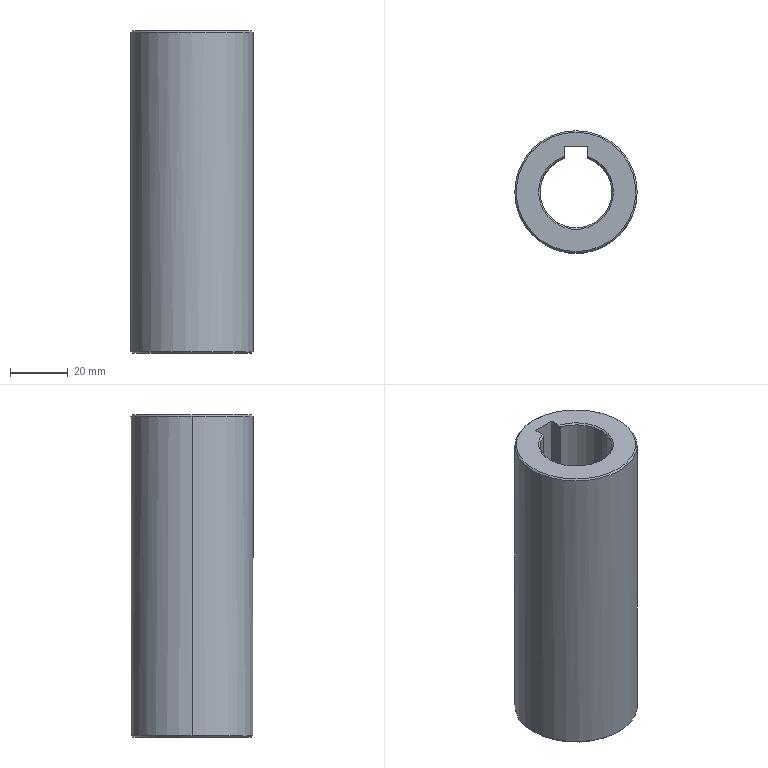Part | STEP file | Output hollow shaft_063_25.step_1 | 1 solid | 18 faces | box 42.5 x 42.5 x 112 mm | volume 100706 mm3 | cone 8 | cylinder 5 | plane 5 | commonest cylinder face diameters 25 x3 42.5 x2
STEP:
#1=CARTESIAN_POINT('',(0.,0.,0.));
#2=DIRECTION('',(0.,0.,1.));
#3=DIRECTION('',(1.,0.,0.));
#4=AXIS2_PLACEMENT_3D('',#1,#2,#3);
#5=CARTESIAN_POINT('',(21.25,0.,-55.5));
#6=VERTEX_POINT('',#5);
#7=CARTESIAN_POINT('',(-21.25,0.,-55.5));
#8=VERTEX_POINT('',#7);
#9=CARTESIAN_POINT('',(0.,0.,-55.5));
#10=DIRECTION('',(0.,0.,1.));
#11=DIRECTION('',(1.,0.,0.));
#12=AXIS2_PLACEMENT_3D('',#9,#10,#11);
#13=CIRCLE('',#12,21.25);
#14=CARTESIAN_POINT('',(0.,0.,92.725));
#15=DIRECTION('',(0.,0.,1.));
#16=DIRECTION('',(1.,0.,0.));
#17=AXIS2_PLACEMENT_3D('',#14,#15,#16);
#18=CYLINDRICAL_SURFACE('',#17,21.25);
#19=CARTESIAN_POINT('',(0.,-148.225));
#20=DIRECTION('',(1.,0.));
#21=VECTOR('',#20,1.);
#22=LINE('',#19,#21);
#23=(GEOMETRIC_REPRESENTATION_CONTEXT(2)PARAMETRIC_REPRESENTATION_CONTEXT()REPRESENTATION_CONTEXT('',''));
#24=DEFINITIONAL_REPRESENTATION('',(#22),#23);
#25=PCURVE('',#18,#24);
#26=CARTESIAN_POINT('',(0.,0.,-55.5));
#27=DIRECTION('',(0.,0.,1.));
#28=DIRECTION('',(1.,0.,0.));
#29=AXIS2_PLACEMENT_3D('',#26,#27,#28);
#30=CONICAL_SURFACE('',#29,21.25,0.7854);
#31=CARTESIAN_POINT('',(0.,0.));
#32=DIRECTION('',(1.,0.));
#33=VECTOR('',#32,1.);
#34=LINE('',#31,#33);
#35=(GEOMETRIC_REPRESENTATION_CONTEXT(2)PARAMETRIC_REPRESENTATION_CONTEXT()REPRESENTATION_CONTEXT('',''));
#36=DEFINITIONAL_REPRESENTATION('',(#34),#35);
#37=PCURVE('',#30,#36);
#38=SURFACE_CURVE('',#13,(#25,#37),.PCURVE_S1.);
#39=EDGE_CURVE('',#6,#8,#38,.T.);
#40=ORIENTED_EDGE('',*,*,#39,.T.);
#41=CARTESIAN_POINT('',(-21.25,0.,55.5));
#42=VERTEX_POINT('',#41);
#43=CARTESIAN_POINT('',(-21.25,0.,92.725));
#44=DIRECTION('',(0.,0.,1.));
#45=VECTOR('',#44,1.);
#46=LINE('',#43,#45);
#47=CARTESIAN_POINT('',(3.142,0.));
#48=DIRECTION('',(0.,1.));
#49=VECTOR('',#48,1.);
#50=LINE('',#47,#49);
#51=(GEOMETRIC_REPRESENTATION_CONTEXT(2)PARAMETRIC_REPRESENTATION_CONTEXT()REPRESENTATION_CONTEXT('',''));
#52=DEFINITIONAL_REPRESENTATION('',(#50),#51);
#53=PCURVE('',#18,#52);
#54=CARTESIAN_POINT('',(0.,0.,92.725));
#55=DIRECTION('',(0.,0.,1.));
#56=DIRECTION('',(1.,0.,0.));
#57=AXIS2_PLACEMENT_3D('',#54,#55,#56);
#58=CYLINDRICAL_SURFACE('',#57,21.25);
#59=CARTESIAN_POINT('',(3.142,0.));
#60=DIRECTION('',(0.,1.));
#61=VECTOR('',#60,1.);
#62=LINE('',#59,#61);
#63=(GEOMETRIC_REPRESENTATION_CONTEXT(2)PARAMETRIC_REPRESENTATION_CONTEXT()REPRESENTATION_CONTEXT('',''));
#64=DEFINITIONAL_REPRESENTATION('',(#62),#63);
#65=PCURVE('',#58,#64);
#66=SURFACE_CURVE('',#46,(#53,#65),.PCURVE_S1.);
#67=EDGE_CURVE('',#8,#42,#66,.T.);
#68=ORIENTED_EDGE('',*,*,#67,.T.);
#69=CARTESIAN_POINT('',(0.,21.25,55.5));
#70=VERTEX_POINT('',#69);
#71=CARTESIAN_POINT('',(0.,0.,55.5));
#72=DIRECTION('',(0.,0.,-1.));
#73=DIRECTION('',(1.,0.,0.));
#74=AXIS2_PLACEMENT_3D('',#71,#72,#73);
#75=CIRCLE('',#74,21.25);
#76=CARTESIAN_POINT('',(6.283,-37.225));
#77=DIRECTION('',(-1.,0.));
#78=VECTOR('',#77,1.);
#79=LINE('',#76,#78);
#80=(GEOMETRIC_REPRESENTATION_CONTEXT(2)PARAMETRIC_REPRESENTATION_CONTEXT()REPRESENTATION_CONTEXT('',''));
#81=DEFINITIONAL_REPRESENTATION('',(#79),#80);
#82=PCURVE('',#18,#81);
#83=CARTESIAN_POINT('',(0.,0.,55.5));
#84=DIRECTION('',(0.,0.,-1.));
#85=DIRECTION('',(0.,1.,0.));
#86=AXIS2_PLACEMENT_3D('',#83,#84,#85);
#87=CONICAL_SURFACE('',#86,21.25,0.7854);
#88=CARTESIAN_POINT('',(1.571,0.));
#89=DIRECTION('',(1.,0.));
#90=VECTOR('',#89,1.);
#91=LINE('',#88,#90);
#92=(GEOMETRIC_REPRESENTATION_CONTEXT(2)PARAMETRIC_REPRESENTATION_CONTEXT()REPRESENTATION_CONTEXT('',''));
#93=DEFINITIONAL_REPRESENTATION('',(#91),#92);
#94=PCURVE('',#87,#93);
#95=SURFACE_CURVE('',#75,(#82,#94),.PCURVE_S1.);
#96=EDGE_CURVE('',#42,#70,#95,.T.);
#97=ORIENTED_EDGE('',*,*,#96,.T.);
#98=CARTESIAN_POINT('',(21.25,0.,55.5));
#99=VERTEX_POINT('',#98);
#100=CARTESIAN_POINT('',(0.,0.,55.5));
#101=DIRECTION('',(0.,0.,-1.));
#102=DIRECTION('',(1.,0.,0.));
#103=AXIS2_PLACEMENT_3D('',#100,#101,#102);
#104=CIRCLE('',#103,21.25);
#105=CARTESIAN_POINT('',(6.283,-37.225));
#106=DIRECTION('',(-1.,0.));
#107=VECTOR('',#106,1.);
#108=LINE('',#105,#107);
#109=(GEOMETRIC_REPRESENTATION_CONTEXT(2)PARAMETRIC_REPRESENTATION_CONTEXT()REPRESENTATION_CONTEXT('',''));
#110=DEFINITIONAL_REPRESENTATION('',(#108),#109);
#111=PCURVE('',#18,#110);
#112=CARTESIAN_POINT('',(0.,0.,55.5));
#113=DIRECTION('',(0.,0.,-1.));
#114=DIRECTION('',(0.,1.,0.));
#115=AXIS2_PLACEMENT_3D('',#112,#113,#114);
#116=CONICAL_SURFACE('',#115,21.25,0.7854);
#117=CARTESIAN_POINT('',(-4.712,0.));
#118=DIRECTION('',(1.,0.));
#119=VECTOR('',#118,1.);
#120=LINE('',#117,#119);
#121=(GEOMETRIC_REPRESENTATION_CONTEXT(2)PARAMETRIC_REPRESENTATION_CONTEXT()REPRESENTATION_CONTEXT('',''));
#122=DEFINITIONAL_REPRESENTATION('',(#120),#121);
#123=PCURVE('',#116,#122);
#124=SURFACE_CURVE('',#104,(#111,#123),.PCURVE_S1.);
#125=EDGE_CURVE('',#70,#99,#124,.T.);
#126=ORIENTED_EDGE('',*,*,#125,.T.);
#127=CARTESIAN_POINT('',(21.25,0.,92.725));
#128=DIRECTION('',(0.,0.,1.));
#129=VECTOR('',#128,1.);
#130=LINE('',#127,#129);
#131=CARTESIAN_POINT('',(0.,0.));
#132=DIRECTION('',(0.,1.));
#133=VECTOR('',#132,1.);
#134=LINE('',#131,#133);
#135=(GEOMETRIC_REPRESENTATION_CONTEXT(2)PARAMETRIC_REPRESENTATION_CONTEXT()REPRESENTATION_CONTEXT('',''));
#136=DEFINITIONAL_REPRESENTATION('',(#134),#135);
#137=PCURVE('',#18,#136);
#138=CARTESIAN_POINT('',(6.283,0.));
#139=DIRECTION('',(0.,1.));
#140=VECTOR('',#139,1.);
#141=LINE('',#138,#140);
#142=(GEOMETRIC_REPRESENTATION_CONTEXT(2)PARAMETRIC_REPRESENTATION_CONTEXT()REPRESENTATION_CONTEXT('',''));
#143=DEFINITIONAL_REPRESENTATION('',(#141),#142);
#144=PCURVE('',#58,#143);
#145=SURFACE_CURVE('',#130,(#137,#144),.PCURVE_S1.);
#146=EDGE_CURVE('',#6,#99,#145,.T.);
#147=ORIENTED_EDGE('',*,*,#146,.F.);
#148=EDGE_LOOP('',(#40,#68,#97,#126,#147));
#149=FACE_BOUND('',#148,.T.);
#150=ADVANCED_FACE('',(#149),#18,.T.);
#151=CARTESIAN_POINT('',(0.,20.75,56.));
#152=VERTEX_POINT('',#151);
#153=CARTESIAN_POINT('',(0.,-20.75,56.));
#154=VERTEX_POINT('',#153);
#155=CARTESIAN_POINT('',(0.,0.,56.));
#156=DIRECTION('',(0.,0.,-1.));
#157=DIRECTION('',(0.,1.,0.));
#158=AXIS2_PLACEMENT_3D('',#155,#156,#157);
#159=CIRCLE('',#158,20.75);
#160=CARTESIAN_POINT('',(0.,-0.5));
#161=DIRECTION('',(1.,0.));
#162=VECTOR('',#161,1.);
#163=LINE('',#160,#162);
#164=(GEOMETRIC_REPRESENTATION_CONTEXT(2)PARAMETRIC_REPRESENTATION_CONTEXT()REPRESENTATION_CONTEXT('',''));
#165=DEFINITIONAL_REPRESENTATION('',(#163),#164);
#166=PCURVE('',#116,#165);
#167=CARTESIAN_POINT('',(0.,13.,56.));
#168=DIRECTION('',(0.,0.,-1.));
#169=DIRECTION('',(-1.,0.,0.));
#170=AXIS2_PLACEMENT_3D('',#167,#168,#169);
#171=PLANE('',#170);
#172=CARTESIAN_POINT('',(0.,-13.));
#173=DIRECTION('',(0.,1.));
#174=AXIS2_PLACEMENT_2D('',#172,#173);
#175=CIRCLE('',#174,20.75);
#176=(GEOMETRIC_REPRESENTATION_CONTEXT(2)PARAMETRIC_REPRESENTATION_CONTEXT()REPRESENTATION_CONTEXT('',''));
#177=DEFINITIONAL_REPRESENTATION('',(#175),#176);
#178=PCURVE('',#171,#177);
#179=SURFACE_CURVE('',#159,(#166,#178),.PCURVE_S1.);
#180=EDGE_CURVE('',#152,#154,#179,.T.);
#181=ORIENTED_EDGE('',*,*,#180,.T.);
#182=CARTESIAN_POINT('',(0.,-21.25,55.5));
#183=VERTEX_POINT('',#182);
#184=CARTESIAN_POINT('',(0.,-21.25,55.5));
#185=DIRECTION('',(0.,-0.7071,-0.7071));
#186=VECTOR('',#185,1.);
#187=LINE('',#184,#186);
#188=CARTESIAN_POINT('',(3.142,0.));
#189=DIRECTION('',(0.,1.));
#190=VECTOR('',#189,1.);
#191=LINE('',#188,#190);
#192=(GEOMETRIC_REPRESENTATION_CONTEXT(2)PARAMETRIC_REPRESENTATION_CONTEXT()REPRESENTATION_CONTEXT('',''));
#193=DEFINITIONAL_REPRESENTATION('',(#191),#192);
#194=PCURVE('',#116,#193);
#195=CARTESIAN_POINT('',(3.142,0.));
#196=DIRECTION('',(0.,1.));
#197=VECTOR('',#196,1.);
#198=LINE('',#195,#197);
#199=(GEOMETRIC_REPRESENTATION_CONTEXT(2)PARAMETRIC_REPRESENTATION_CONTEXT()REPRESENTATION_CONTEXT('',''));
#200=DEFINITIONAL_REPRESENTATION('',(#198),#199);
#201=PCURVE('',#87,#200);
#202=SURFACE_CURVE('',#187,(#194,#201),.PCURVE_S1.);
#203=EDGE_CURVE('',#154,#183,#202,.T.);
#204=ORIENTED_EDGE('',*,*,#203,.T.);
#205=CARTESIAN_POINT('',(0.,0.,55.5));
#206=DIRECTION('',(0.,0.,-1.));
#207=DIRECTION('',(1.,0.,0.));
#208=AXIS2_PLACEMENT_3D('',#205,#206,#207);
#209=CIRCLE('',#208,21.25);
#210=CARTESIAN_POINT('',(1.571,0.));
#211=DIRECTION('',(1.,0.));
#212=VECTOR('',#211,1.);
#213=LINE('',#210,#212);
#214=(GEOMETRIC_REPRESENTATION_CONTEXT(2)PARAMETRIC_REPRESENTATION_CONTEXT()REPRESENTATION_CONTEXT('',''));
#215=DEFINITIONAL_REPRESENTATION('',(#213),#214);
#216=PCURVE('',#116,#215);
#217=CARTESIAN_POINT('',(6.283,-37.225));
#218=DIRECTION('',(-1.,0.));
#219=VECTOR('',#218,1.);
#220=LINE('',#217,#219);
#221=(GEOMETRIC_REPRESENTATION_CONTEXT(2)PARAMETRIC_REPRESENTATION_CONTEXT()REPRESENTATION_CONTEXT('',''));
#222=DEFINITIONAL_REPRESENTATION('',(#220),#221);
#223=PCURVE('',#58,#222);
#224=SURFACE_CURVE('',#209,(#216,#223),.PCURVE_S1.);
#225=EDGE_CURVE('',#99,#183,#224,.T.);
#226=ORIENTED_EDGE('',*,*,#225,.F.);
#227=ORIENTED_EDGE('',*,*,#125,.F.);
#228=CARTESIAN_POINT('',(0.,21.25,55.5));
#229=DIRECTION('',(0.,0.7071,-0.7071));
#230=VECTOR('',#229,1.);
#231=LINE('',#228,#230);
#232=CARTESIAN_POINT('',(0.,0.));
#233=DIRECTION('',(0.,1.));
#234=VECTOR('',#233,1.);
#235=LINE('',#232,#234);
#236=(GEOMETRIC_REPRESENTATION_CONTEXT(2)PARAMETRIC_REPRESENTATION_CONTEXT()REPRESENTATION_CONTEXT('',''));
#237=DEFINITIONAL_REPRESENTATION('',(#235),#236);
#238=PCURVE('',#116,#237);
#239=CARTESIAN_POINT('',(6.283,0.));
#240=DIRECTION('',(0.,1.));
#241=VECTOR('',#240,1.);
#242=LINE('',#239,#241);
#243=(GEOMETRIC_REPRESENTATION_CONTEXT(2)PARAMETRIC_REPRESENTATION_CONTEXT()REPRESENTATION_CONTEXT('',''));
#244=DEFINITIONAL_REPRESENTATION('',(#242),#243);
#245=PCURVE('',#87,#244);
#246=SURFACE_CURVE('',#231,(#238,#245),.PCURVE_S1.);
#247=EDGE_CURVE('',#152,#70,#246,.T.);
#248=ORIENTED_EDGE('',*,*,#247,.F.);
#249=EDGE_LOOP('',(#181,#204,#226,#227,#248));
#250=FACE_BOUND('',#249,.T.);
#251=ADVANCED_FACE('',(#250),#116,.T.);
#252=CARTESIAN_POINT('',(20.75,0.,-56.));
#253=VERTEX_POINT('',#252);
#254=CARTESIAN_POINT('',(-20.75,0.,-56.));
#255=VERTEX_POINT('',#254);
#256=CARTESIAN_POINT('',(0.,0.,-56.));
#257=DIRECTION('',(0.,0.,1.));
#258=DIRECTION('',(1.,0.,0.));
#259=AXIS2_PLACEMENT_3D('',#256,#257,#258);
#260=CIRCLE('',#259,20.75);
#261=CARTESIAN_POINT('',(0.,-0.5));
#262=DIRECTION('',(1.,0.));
#263=VECTOR('',#262,1.);
#264=LINE('',#261,#263);
#265=(GEOMETRIC_REPRESENTATION_CONTEXT(2)PARAMETRIC_REPRESENTATION_CONTEXT()REPRESENTATION_CONTEXT('',''));
#266=DEFINITIONAL_REPRESENTATION('',(#264),#265);
#267=PCURVE('',#30,#266);
#268=CARTESIAN_POINT('',(0.,20.75,-56.));
#269=DIRECTION('',(0.,0.,1.));
#270=DIRECTION('',(1.,0.,0.));
#271=AXIS2_PLACEMENT_3D('',#268,#269,#270);
#272=PLANE('',#271);
#273=CARTESIAN_POINT('',(0.,-20.75));
#274=DIRECTION('',(1.,0.));
#275=AXIS2_PLACEMENT_2D('',#273,#274);
#276=CIRCLE('',#275,20.75);
#277=(GEOMETRIC_REPRESENTATION_CONTEXT(2)PARAMETRIC_REPRESENTATION_CONTEXT()REPRESENTATION_CONTEXT('',''));
#278=DEFINITIONAL_REPRESENTATION('',(#276),#277);
#279=PCURVE('',#272,#278);
#280=SURFACE_CURVE('',#260,(#267,#279),.PCURVE_S1.);
#281=EDGE_CURVE('',#253,#255,#280,.T.);
#282=ORIENTED_EDGE('',*,*,#281,.T.);
#283=CARTESIAN_POINT('',(-21.25,0.,-55.5));
#284=DIRECTION('',(-0.7071,0.,0.7071));
#285=VECTOR('',#284,1.);
#286=LINE('',#283,#285);
#287=CARTESIAN_POINT('',(3.142,0.));
#288=DIRECTION('',(0.,1.));
#289=VECTOR('',#288,1.);
#290=LINE('',#287,#289);
#291=(GEOMETRIC_REPRESENTATION_CONTEXT(2)PARAMETRIC_REPRESENTATION_CONTEXT()REPRESENTATION_CONTEXT('',''));
#292=DEFINITIONAL_REPRESENTATION('',(#290),#291);
#293=PCURVE('',#30,#292);
#294=CARTESIAN_POINT('',(0.,0.,-55.5));
#295=DIRECTION('',(0.,0.,1.));
#296=DIRECTION('',(1.,0.,0.));
#297=AXIS2_PLACEMENT_3D('',#294,#295,#296);
#298=CONICAL_SURFACE('',#297,21.25,0.7854);
#299=CARTESIAN_POINT('',(3.142,0.));
#300=DIRECTION('',(0.,1.));
#301=VECTOR('',#300,1.);
#302=LINE('',#299,#301);
#303=(GEOMETRIC_REPRESENTATION_CONTEXT(2)PARAMETRIC_REPRESENTATION_CONTEXT()REPRESENTATION_CONTEXT('',''));
#304=DEFINITIONAL_REPRESENTATION('',(#302),#303);
#305=PCURVE('',#298,#304);
#306=SURFACE_CURVE('',#286,(#293,#305),.PCURVE_S1.);
#307=EDGE_CURVE('',#255,#8,#306,.T.);
#308=ORIENTED_EDGE('',*,*,#307,.T.);
#309=ORIENTED_EDGE('',*,*,#39,.F.);
#310=CARTESIAN_POINT('',(21.25,0.,-55.5));
#311=DIRECTION('',(0.7071,0.,0.7071));
#312=VECTOR('',#311,1.);
#313=LINE('',#310,#312);
#314=CARTESIAN_POINT('',(0.,0.));
#315=DIRECTION('',(0.,1.));
#316=VECTOR('',#315,1.);
#317=LINE('',#314,#316);
#318=(GEOMETRIC_REPRESENTATION_CONTEXT(2)PARAMETRIC_REPRESENTATION_CONTEXT()REPRESENTATION_CONTEXT('',''));
#319=DEFINITIONAL_REPRESENTATION('',(#317),#318);
#320=PCURVE('',#30,#319);
#321=CARTESIAN_POINT('',(6.283,0.));
#322=DIRECTION('',(0.,1.));
#323=VECTOR('',#322,1.);
#324=LINE('',#321,#323);
#325=(GEOMETRIC_REPRESENTATION_CONTEXT(2)PARAMETRIC_REPRESENTATION_CONTEXT()REPRESENTATION_CONTEXT('',''));
#326=DEFINITIONAL_REPRESENTATION('',(#324),#325);
#327=PCURVE('',#298,#326);
#328=SURFACE_CURVE('',#313,(#320,#327),.PCURVE_S1.);
#329=EDGE_CURVE('',#253,#6,#328,.T.);
#330=ORIENTED_EDGE('',*,*,#329,.F.);
#331=EDGE_LOOP('',(#282,#308,#309,#330));
#332=FACE_BOUND('',#331,.T.);
#333=ADVANCED_FACE('',(#332),#30,.T.);
#334=CARTESIAN_POINT('',(12.5,0.,55.5));
#335=VERTEX_POINT('',#334);
#336=CARTESIAN_POINT('',(13.,0.,56.));
#337=VERTEX_POINT('',#336);
#338=CARTESIAN_POINT('',(13.,0.,56.));
#339=DIRECTION('',(0.7071,0.,0.7071));
#340=VECTOR('',#339,1.);
#341=LINE('',#338,#340);
#342=CARTESIAN_POINT('',(0.,0.,56.));
#343=DIRECTION('',(0.,0.,1.));
#344=DIRECTION('',(1.,0.,0.));
#345=AXIS2_PLACEMENT_3D('',#342,#343,#344);
#346=CONICAL_SURFACE('',#345,13.,0.7854);
#347=CARTESIAN_POINT('',(6.283,0.));
#348=DIRECTION('',(0.,1.));
#349=VECTOR('',#348,1.);
#350=LINE('',#347,#349);
#351=(GEOMETRIC_REPRESENTATION_CONTEXT(2)PARAMETRIC_REPRESENTATION_CONTEXT()REPRESENTATION_CONTEXT('',''));
#352=DEFINITIONAL_REPRESENTATION('',(#350),#351);
#353=PCURVE('',#346,#352);
#354=CARTESIAN_POINT('',(0.,0.,56.));
#355=DIRECTION('',(0.,0.,1.));
#356=DIRECTION('',(1.,0.,0.));
#357=AXIS2_PLACEMENT_3D('',#354,#355,#356);
#358=CONICAL_SURFACE('',#357,13.,0.7854);
#359=CARTESIAN_POINT('',(0.,0.));
#360=DIRECTION('',(0.,1.));
#361=VECTOR('',#360,1.);
#362=LINE('',#359,#361);
#363=(GEOMETRIC_REPRESENTATION_CONTEXT(2)PARAMETRIC_REPRESENTATION_CONTEXT()REPRESENTATION_CONTEXT('',''));
#364=DEFINITIONAL_REPRESENTATION('',(#362),#363);
#365=PCURVE('',#358,#364);
#366=SURFACE_CURVE('',#341,(#353,#365),.PCURVE_S1.);
#367=EDGE_CURVE('',#335,#337,#366,.T.);
#368=ORIENTED_EDGE('',*,*,#367,.T.);
#369=CARTESIAN_POINT('',(-13.,0.,56.));
#370=VERTEX_POINT('',#369);
#371=CARTESIAN_POINT('',(0.,0.,56.));
#372=DIRECTION('',(0.,0.,1.));
#373=DIRECTION('',(1.,0.,0.));
#374=AXIS2_PLACEMENT_3D('',#371,#372,#373);
#375=CIRCLE('',#374,13.);
#376=CARTESIAN_POINT('',(0.,0.));
#377=DIRECTION('',(1.,0.));
#378=VECTOR('',#377,1.);
#379=LINE('',#376,#378);
#380=(GEOMETRIC_REPRESENTATION_CONTEXT(2)PARAMETRIC_REPRESENTATION_CONTEXT()REPRESENTATION_CONTEXT('',''));
#381=DEFINITIONAL_REPRESENTATION('',(#379),#380);
#382=PCURVE('',#346,#381);
#383=CARTESIAN_POINT('',(-13.,-13.));
#384=CARTESIAN_POINT('',(-13.,9.517));
#385=CARTESIAN_POINT('',(6.5,-1.742));
#386=CARTESIAN_POINT('',(26.,-13.));
#387=CARTESIAN_POINT('',(6.5,-24.258));
#388=CARTESIAN_POINT('',(-13.,-35.517));
#389=CARTESIAN_POINT('',(-13.,-13.));
#390=(BOUNDED_CURVE()B_SPLINE_CURVE(2,(#383,#384,#385,#386,#387,#388,#389),.UNSPECIFIED.,.T.,.F.)B_SPLINE_CURVE_WITH_KNOTS((1,2,2,2,2,1),(-2.094,0.,2.094,4.189,6.283,8.378),.UNSPECIFIED.)CURVE()GEOMETRIC_REPRESENTATION_ITEM()RATIONAL_B_SPLINE_CURVE((1.,0.5,1.,0.5,1.,0.5,1.))REPRESENTATION_ITEM(''));
#391=(GEOMETRIC_REPRESENTATION_CONTEXT(2)PARAMETRIC_REPRESENTATION_CONTEXT()REPRESENTATION_CONTEXT('',''));
#392=DEFINITIONAL_REPRESENTATION('',(#390),#391);
#393=PCURVE('',#171,#392);
#394=SURFACE_CURVE('',#375,(#382,#393),.PCURVE_S1.);
#395=EDGE_CURVE('',#370,#337,#394,.T.);
#396=ORIENTED_EDGE('',*,*,#395,.F.);
#397=CARTESIAN_POINT('',(-12.5,0.,55.5));
#398=VERTEX_POINT('',#397);
#399=CARTESIAN_POINT('',(-13.,0.,56.));
#400=DIRECTION('',(-0.7071,0.,0.7071));
#401=VECTOR('',#400,1.);
#402=LINE('',#399,#401);
#403=CARTESIAN_POINT('',(3.142,0.));
#404=DIRECTION('',(0.,1.));
#405=VECTOR('',#404,1.);
#406=LINE('',#403,#405);
#407=(GEOMETRIC_REPRESENTATION_CONTEXT(2)PARAMETRIC_REPRESENTATION_CONTEXT()REPRESENTATION_CONTEXT('',''));
#408=DEFINITIONAL_REPRESENTATION('',(#406),#407);
#409=PCURVE('',#346,#408);
#410=CARTESIAN_POINT('',(0.,0.,56.));
#411=DIRECTION('',(0.,0.,1.));
#412=DIRECTION('',(1.,0.,0.));
#413=AXIS2_PLACEMENT_3D('',#410,#411,#412);
#414=CONICAL_SURFACE('',#413,13.,0.7854);
#415=CARTESIAN_POINT('',(3.142,0.));
#416=DIRECTION('',(0.,1.));
#417=VECTOR('',#416,1.);
#418=LINE('',#415,#417);
#419=(GEOMETRIC_REPRESENTATION_CONTEXT(2)PARAMETRIC_REPRESENTATION_CONTEXT()REPRESENTATION_CONTEXT('',''));
#420=DEFINITIONAL_REPRESENTATION('',(#418),#419);
#421=PCURVE('',#414,#420);
#422=SURFACE_CURVE('',#402,(#409,#421),.PCURVE_S1.);
#423=EDGE_CURVE('',#398,#370,#422,.T.);
#424=ORIENTED_EDGE('',*,*,#423,.F.);
#425=CARTESIAN_POINT('',(0.,0.,55.5));
#426=DIRECTION('',(0.,0.,1.));
#427=DIRECTION('',(1.,0.,0.));
#428=AXIS2_PLACEMENT_3D('',#425,#426,#427);
#429=CIRCLE('',#428,12.5);
#430=CARTESIAN_POINT('',(0.,-0.5));
#431=DIRECTION('',(1.,0.));
#432=VECTOR('',#431,1.);
#433=LINE('',#430,#432);
#434=(GEOMETRIC_REPRESENTATION_CONTEXT(2)PARAMETRIC_REPRESENTATION_CONTEXT()REPRESENTATION_CONTEXT('',''));
#435=DEFINITIONAL_REPRESENTATION('',(#433),#434);
#436=PCURVE('',#346,#435);
#437=CARTESIAN_POINT('',(0.,0.,92.725));
#438=DIRECTION('',(0.,0.,1.));
#439=DIRECTION('',(1.,0.,0.));
#440=AXIS2_PLACEMENT_3D('',#437,#438,#439);
#441=CYLINDRICAL_SURFACE('',#440,12.5);
#442=CARTESIAN_POINT('',(0.,-37.225));
#443=DIRECTION('',(1.,0.));
#444=VECTOR('',#443,1.);
#445=LINE('',#442,#444);
#446=(GEOMETRIC_REPRESENTATION_CONTEXT(2)PARAMETRIC_REPRESENTATION_CONTEXT()REPRESENTATION_CONTEXT('',''));
#447=DEFINITIONAL_REPRESENTATION('',(#445),#446);
#448=PCURVE('',#441,#447);
#449=SURFACE_CURVE('',#429,(#436,#448),.PCURVE_S1.);
#450=EDGE_CURVE('',#398,#335,#449,.T.);
#451=ORIENTED_EDGE('',*,*,#450,.T.);
#452=EDGE_LOOP('',(#368,#396,#424,#451));
#453=FACE_BOUND('',#452,.F.);
#454=ADVANCED_FACE('',(#453),#346,.F.);
#455=CARTESIAN_POINT('',(4.,12.369,56.));
#456=VERTEX_POINT('',#455);
#457=CARTESIAN_POINT('',(4.,11.843,55.5));
#458=VERTEX_POINT('',#457);
#459=CARTESIAN_POINT('',(4.,12.369,56.));
#460=CARTESIAN_POINT('',(4.,12.194,55.833));
#461=CARTESIAN_POINT('',(4.,12.018,55.666));
#462=CARTESIAN_POINT('',(4.,11.843,55.5));
#463=B_SPLINE_CURVE_WITH_KNOTS('',3,(#459,#460,#461,#462),.UNSPECIFIED.,.F.,.F.,(4,4),(0.,0.0007262),.PIECEWISE_BEZIER_KNOTS.);
#464=CARTESIAN_POINT('',(1.258,0.));
#465=CARTESIAN_POINT('',(1.258,-0.007584));
#466=CARTESIAN_POINT('',(1.257,-0.02275));
#467=CARTESIAN_POINT('',(1.257,-0.0455));
#468=CARTESIAN_POINT('',(1.256,-0.06825));
#469=CARTESIAN_POINT('',(1.256,-0.09099));
#470=CARTESIAN_POINT('',(1.255,-0.1137));
#471=CARTESIAN_POINT('',(1.255,-0.1365));
#472=CARTESIAN_POINT('',(1.254,-0.1592));
#473=CARTESIAN_POINT('',(1.253,-0.1819));
#474=CARTESIAN_POINT('',(1.253,-0.2047));
#475=CARTESIAN_POINT('',(1.252,-0.2274));
#476=CARTESIAN_POINT('',(1.252,-0.2501));
#477=CARTESIAN_POINT('',(1.251,-0.2729));
#478=CARTESIAN_POINT('',(1.25,-0.2956));
#479=CARTESIAN_POINT('',(1.25,-0.3183));
#480=CARTESIAN_POINT('',(1.249,-0.341));
#481=CARTESIAN_POINT('',(1.249,-0.3637));
#482=CARTESIAN_POINT('',(1.248,-0.3865));
#483=CARTESIAN_POINT('',(1.248,-0.4092));
#484=CARTESIAN_POINT('',(1.247,-0.4319));
#485=CARTESIAN_POINT('',(1.246,-0.4546));
#486=CARTESIAN_POINT('',(1.246,-0.4773));
#487=CARTESIAN_POINT('',(1.245,-0.4924));
#488=CARTESIAN_POINT('',(1.245,-0.5));
#489=B_SPLINE_CURVE_WITH_KNOTS('',3,(#464,#465,#466,#467,#468,#469,#470,#471,#472,#473,#474,#475,#476,#477,#478,#479,#480,#481,#482,#483,#484,#485,#486,#487,#488),.UNSPECIFIED.,.F.,.F.,(4,1,1,1,1,1,1,1,1,1,1,1,1,1,1,1,1,1,1,1,1,1,4),(0.,0.00003301,0.00006601,0.00009902,0.000132,0.000165,0.000198,0.0002311,0.0002641,0.0002971,0.0003301,0.0003631,0.0003961,0.0004291,0.0004621,0.0004951,0.0005281,0.0005611,0.0005941,0.0006271,0.0006601,0.0006932,0.0007262),.QUASI_UNIFORM_KNOTS.);
#490=(GEOMETRIC_REPRESENTATION_CONTEXT(2)PARAMETRIC_REPRESENTATION_CONTEXT()REPRESENTATION_CONTEXT('',''));
#491=DEFINITIONAL_REPRESENTATION('',(#489),#490);
#492=PCURVE('',#358,#491);
#493=CARTESIAN_POINT('',(4.,11.843,-56.));
#494=DIRECTION('',(1.,0.,0.));
#495=DIRECTION('',(0.,1.,0.));
#496=AXIS2_PLACEMENT_3D('',#493,#494,#495);
#497=PLANE('',#496);
#498=CARTESIAN_POINT('',(0.5266,112.));
#499=CARTESIAN_POINT('',(0.3512,111.833));
#500=CARTESIAN_POINT('',(0.1757,111.666));
#501=CARTESIAN_POINT('',(0.,111.5));
#502=B_SPLINE_CURVE_WITH_KNOTS('',3,(#498,#499,#500,#501),.UNSPECIFIED.,.F.,.F.,(4,4),(0.,0.0007262),.PIECEWISE_BEZIER_KNOTS.);
#503=(GEOMETRIC_REPRESENTATION_CONTEXT(2)PARAMETRIC_REPRESENTATION_CONTEXT()REPRESENTATION_CONTEXT('',''));
#504=DEFINITIONAL_REPRESENTATION('',(#502),#503);
#505=PCURVE('',#497,#504);
#506=SURFACE_CURVE('',#463,(#492,#505),.PCURVE_S1.);
#507=EDGE_CURVE('',#456,#458,#506,.T.);
#508=ORIENTED_EDGE('',*,*,#507,.F.);
#509=CARTESIAN_POINT('',(0.,0.,56.));
#510=DIRECTION('',(0.,0.,1.));
#511=DIRECTION('',(1.,0.,0.));
#512=AXIS2_PLACEMENT_3D('',#509,#510,#511);
#513=CIRCLE('',#512,13.);
#514=CARTESIAN_POINT('',(0.,0.));
#515=DIRECTION('',(1.,0.));
#516=VECTOR('',#515,1.);
#517=LINE('',#514,#516);
#518=(GEOMETRIC_REPRESENTATION_CONTEXT(2)PARAMETRIC_REPRESENTATION_CONTEXT()REPRESENTATION_CONTEXT('',''));
#519=DEFINITIONAL_REPRESENTATION('',(#517),#518);
#520=PCURVE('',#358,#519);
#521=CARTESIAN_POINT('',(-13.,-13.));
#522=CARTESIAN_POINT('',(-13.,9.517));
#523=CARTESIAN_POINT('',(6.5,-1.742));
#524=CARTESIAN_POINT('',(26.,-13.));
#525=CARTESIAN_POINT('',(6.5,-24.258));
#526=CARTESIAN_POINT('',(-13.,-35.517));
#527=CARTESIAN_POINT('',(-13.,-13.));
#528=(BOUNDED_CURVE()B_SPLINE_CURVE(2,(#521,#522,#523,#524,#525,#526,#527),.UNSPECIFIED.,.T.,.F.)B_SPLINE_CURVE_WITH_KNOTS((1,2,2,2,2,1),(-2.094,0.,2.094,4.189,6.283,8.378),.UNSPECIFIED.)CURVE()GEOMETRIC_REPRESENTATION_ITEM()RATIONAL_B_SPLINE_CURVE((1.,0.5,1.,0.5,1.,0.5,1.))REPRESENTATION_ITEM(''));
#529=(GEOMETRIC_REPRESENTATION_CONTEXT(2)PARAMETRIC_REPRESENTATION_CONTEXT()REPRESENTATION_CONTEXT('',''));
#530=DEFINITIONAL_REPRESENTATION('',(#528),#529);
#531=PCURVE('',#171,#530);
#532=SURFACE_CURVE('',#513,(#520,#531),.PCURVE_S1.);
#533=EDGE_CURVE('',#337,#456,#532,.T.);
#534=ORIENTED_EDGE('',*,*,#533,.F.);
#535=ORIENTED_EDGE('',*,*,#367,.F.);
#536=CARTESIAN_POINT('',(0.,0.,55.5));
#537=DIRECTION('',(0.,0.,1.));
#538=DIRECTION('',(1.,0.,0.));
#539=AXIS2_PLACEMENT_3D('',#536,#537,#538);
#540=CIRCLE('',#539,12.5);
#541=CARTESIAN_POINT('',(0.,-0.5));
#542=DIRECTION('',(1.,0.));
#543=VECTOR('',#542,1.);
#544=LINE('',#541,#543);
#545=(GEOMETRIC_REPRESENTATION_CONTEXT(2)PARAMETRIC_REPRESENTATION_CONTEXT()REPRESENTATION_CONTEXT('',''));
#546=DEFINITIONAL_REPRESENTATION('',(#544),#545);
#547=PCURVE('',#358,#546);
#548=CARTESIAN_POINT('',(0.,0.,92.725));
#549=DIRECTION('',(0.,0.,1.));
#550=DIRECTION('',(1.,0.,0.));
#551=AXIS2_PLACEMENT_3D('',#548,#549,#550);
#552=CYLINDRICAL_SURFACE('',#551,12.5);
#553=CARTESIAN_POINT('',(0.,-37.225));
#554=DIRECTION('',(1.,0.));
#555=VECTOR('',#554,1.);
#556=LINE('',#553,#555);
#557=(GEOMETRIC_REPRESENTATION_CONTEXT(2)PARAMETRIC_REPRESENTATION_CONTEXT()REPRESENTATION_CONTEXT('',''));
#558=DEFINITIONAL_REPRESENTATION('',(#556),#557);
#559=PCURVE('',#552,#558);
#560=SURFACE_CURVE('',#540,(#547,#559),.PCURVE_S1.);
#561=EDGE_CURVE('',#335,#458,#560,.T.);
#562=ORIENTED_EDGE('',*,*,#561,.T.);
#563=EDGE_LOOP('',(#508,#534,#535,#562));
#564=FACE_BOUND('',#563,.F.);
#565=ADVANCED_FACE('',(#564),#358,.F.);
#566=CARTESIAN_POINT('',(12.5,0.,-55.5));
#567=VERTEX_POINT('',#566);
#568=CARTESIAN_POINT('',(12.5,0.,92.725));
#569=DIRECTION('',(0.,0.,1.));
#570=VECTOR('',#569,1.);
#571=LINE('',#568,#570);
#572=CARTESIAN_POINT('',(6.283,0.));
#573=DIRECTION('',(0.,1.));
#574=VECTOR('',#573,1.);
#575=LINE('',#572,#574);
#576=(GEOMETRIC_REPRESENTATION_CONTEXT(2)PARAMETRIC_REPRESENTATION_CONTEXT()REPRESENTATION_CONTEXT('',''));
#577=DEFINITIONAL_REPRESENTATION('',(#575),#576);
#578=PCURVE('',#441,#577);
#579=CARTESIAN_POINT('',(0.,0.));
#580=DIRECTION('',(0.,1.));
#581=VECTOR('',#580,1.);
#582=LINE('',#579,#581);
#583=(GEOMETRIC_REPRESENTATION_CONTEXT(2)PARAMETRIC_REPRESENTATION_CONTEXT()REPRESENTATION_CONTEXT('',''));
#584=DEFINITIONAL_REPRESENTATION('',(#582),#583);
#585=PCURVE('',#552,#584);
#586=SURFACE_CURVE('',#571,(#578,#585),.PCURVE_S1.);
#587=EDGE_CURVE('',#567,#335,#586,.T.);
#588=ORIENTED_EDGE('',*,*,#587,.T.);
#589=ORIENTED_EDGE('',*,*,#450,.F.);
#590=CARTESIAN_POINT('',(-12.5,0.,-55.5));
#591=VERTEX_POINT('',#590);
#592=CARTESIAN_POINT('',(-12.5,0.,92.725));
#593=DIRECTION('',(0.,0.,1.));
#594=VECTOR('',#593,1.);
#595=LINE('',#592,#594);
#596=CARTESIAN_POINT('',(3.142,0.));
#597=DIRECTION('',(0.,1.));
#598=VECTOR('',#597,1.);
#599=LINE('',#596,#598);
#600=(GEOMETRIC_REPRESENTATION_CONTEXT(2)PARAMETRIC_REPRESENTATION_CONTEXT()REPRESENTATION_CONTEXT('',''));
#601=DEFINITIONAL_REPRESENTATION('',(#599),#600);
#602=PCURVE('',#441,#601);
#603=CARTESIAN_POINT('',(0.,0.,92.725));
#604=DIRECTION('',(0.,0.,1.));
#605=DIRECTION('',(1.,0.,0.));
#606=AXIS2_PLACEMENT_3D('',#603,#604,#605);
#607=CYLINDRICAL_SURFACE('',#606,12.5);
#608=CARTESIAN_POINT('',(3.142,0.));
#609=DIRECTION('',(0.,1.));
#610=VECTOR('',#609,1.);
#611=LINE('',#608,#610);
#612=(GEOMETRIC_REPRESENTATION_CONTEXT(2)PARAMETRIC_REPRESENTATION_CONTEXT()REPRESENTATION_CONTEXT('',''));
#613=DEFINITIONAL_REPRESENTATION('',(#611),#612);
#614=PCURVE('',#607,#613);
#615=SURFACE_CURVE('',#595,(#602,#614),.PCURVE_S1.);
#616=EDGE_CURVE('',#591,#398,#615,.T.);
#617=ORIENTED_EDGE('',*,*,#616,.F.);
#618=CARTESIAN_POINT('',(0.,0.,-55.5));
#619=DIRECTION('',(0.,0.,-1.));
#620=DIRECTION('',(-1.,0.,0.));
#621=AXIS2_PLACEMENT_3D('',#618,#619,#620);
#622=CIRCLE('',#621,12.5);
#623=CARTESIAN_POINT('',(9.425,-148.225));
#624=DIRECTION('',(-1.,0.));
#625=VECTOR('',#624,1.);
#626=LINE('',#623,#625);
#627=(GEOMETRIC_REPRESENTATION_CONTEXT(2)PARAMETRIC_REPRESENTATION_CONTEXT()REPRESENTATION_CONTEXT('',''));
#628=DEFINITIONAL_REPRESENTATION('',(#626),#627);
#629=PCURVE('',#441,#628);
#630=CARTESIAN_POINT('',(0.,0.,-56.));
#631=DIRECTION('',(0.,0.,-1.));
#632=DIRECTION('',(0.,1.,0.));
#633=AXIS2_PLACEMENT_3D('',#630,#631,#632);
#634=CONICAL_SURFACE('',#633,13.,0.7854);
#635=CARTESIAN_POINT('',(-1.571,-0.5));
#636=DIRECTION('',(1.,0.));
#637=VECTOR('',#636,1.);
#638=LINE('',#635,#637);
#639=(GEOMETRIC_REPRESENTATION_CONTEXT(2)PARAMETRIC_REPRESENTATION_CONTEXT()REPRESENTATION_CONTEXT('',''));
#640=DEFINITIONAL_REPRESENTATION('',(#638),#639);
#641=PCURVE('',#634,#640);
#642=SURFACE_CURVE('',#622,(#629,#641),.PCURVE_S1.);
#643=EDGE_CURVE('',#567,#591,#642,.T.);
#644=ORIENTED_EDGE('',*,*,#643,.F.);
#645=EDGE_LOOP('',(#588,#589,#617,#644));
#646=FACE_BOUND('',#645,.F.);
#647=ADVANCED_FACE('',(#646),#441,.F.);
#648=CARTESIAN_POINT('',(4.,11.843,-55.5));
#649=VERTEX_POINT('',#648);
#650=CARTESIAN_POINT('',(4.,11.843,-56.));
#651=DIRECTION('',(0.,0.,-1.));
#652=VECTOR('',#651,1.);
#653=LINE('',#650,#652);
#654=CARTESIAN_POINT('',(1.245,-148.725));
#655=DIRECTION('',(0.,-1.));
#656=VECTOR('',#655,1.);
#657=LINE('',#654,#656);
#658=(GEOMETRIC_REPRESENTATION_CONTEXT(2)PARAMETRIC_REPRESENTATION_CONTEXT()REPRESENTATION_CONTEXT('',''));
#659=DEFINITIONAL_REPRESENTATION('',(#657),#658);
#660=PCURVE('',#552,#659);
#661=CARTESIAN_POINT('',(0.,0.));
#662=DIRECTION('',(0.,-1.));
#663=VECTOR('',#662,1.);
#664=LINE('',#661,#663);
#665=(GEOMETRIC_REPRESENTATION_CONTEXT(2)PARAMETRIC_REPRESENTATION_CONTEXT()REPRESENTATION_CONTEXT('',''));
#666=DEFINITIONAL_REPRESENTATION('',(#664),#665);
#667=PCURVE('',#497,#666);
#668=SURFACE_CURVE('',#653,(#660,#667),.PCURVE_S1.);
#669=EDGE_CURVE('',#458,#649,#668,.T.);
#670=ORIENTED_EDGE('',*,*,#669,.F.);
#671=ORIENTED_EDGE('',*,*,#561,.F.);
#672=ORIENTED_EDGE('',*,*,#587,.F.);
#673=CARTESIAN_POINT('',(0.,0.,-55.5));
#674=DIRECTION('',(0.,0.,-1.));
#675=DIRECTION('',(-1.,0.,0.));
#676=AXIS2_PLACEMENT_3D('',#673,#674,#675);
#677=CIRCLE('',#676,12.5);
#678=CARTESIAN_POINT('',(3.142,-148.225));
#679=DIRECTION('',(-1.,0.));
#680=VECTOR('',#679,1.);
#681=LINE('',#678,#680);
#682=(GEOMETRIC_REPRESENTATION_CONTEXT(2)PARAMETRIC_REPRESENTATION_CONTEXT()REPRESENTATION_CONTEXT('',''));
#683=DEFINITIONAL_REPRESENTATION('',(#681),#682);
#684=PCURVE('',#552,#683);
#685=CARTESIAN_POINT('',(-1.571,-0.5));
#686=DIRECTION('',(1.,0.));
#687=VECTOR('',#686,1.);
#688=LINE('',#685,#687);
#689=(GEOMETRIC_REPRESENTATION_CONTEXT(2)PARAMETRIC_REPRESENTATION_CONTEXT()REPRESENTATION_CONTEXT('',''));
#690=DEFINITIONAL_REPRESENTATION('',(#688),#689);
#691=PCURVE('',#634,#690);
#692=SURFACE_CURVE('',#677,(#684,#691),.PCURVE_S1.);
#693=EDGE_CURVE('',#649,#567,#692,.T.);
#694=ORIENTED_EDGE('',*,*,#693,.F.);
#695=EDGE_LOOP('',(#670,#671,#672,#694));
#696=FACE_BOUND('',#695,.F.);
#697=ADVANCED_FACE('',(#696),#552,.F.);
#698=ORIENTED_EDGE('',*,*,#67,.F.);
#699=CARTESIAN_POINT('',(0.,0.,-55.5));
#700=DIRECTION('',(0.,0.,1.));
#701=DIRECTION('',(1.,0.,0.));
#702=AXIS2_PLACEMENT_3D('',#699,#700,#701);
#703=CIRCLE('',#702,21.25);
#704=CARTESIAN_POINT('',(0.,-148.225));
#705=DIRECTION('',(1.,0.));
#706=VECTOR('',#705,1.);
#707=LINE('',#704,#706);
#708=(GEOMETRIC_REPRESENTATION_CONTEXT(2)PARAMETRIC_REPRESENTATION_CONTEXT()REPRESENTATION_CONTEXT('',''));
#709=DEFINITIONAL_REPRESENTATION('',(#707),#708);
#710=PCURVE('',#58,#709);
#711=CARTESIAN_POINT('',(0.,0.));
#712=DIRECTION('',(1.,0.));
#713=VECTOR('',#712,1.);
#714=LINE('',#711,#713);
#715=(GEOMETRIC_REPRESENTATION_CONTEXT(2)PARAMETRIC_REPRESENTATION_CONTEXT()REPRESENTATION_CONTEXT('',''));
#716=DEFINITIONAL_REPRESENTATION('',(#714),#715);
#717=PCURVE('',#298,#716);
#718=SURFACE_CURVE('',#703,(#710,#717),.PCURVE_S1.);
#719=EDGE_CURVE('',#8,#6,#718,.T.);
#720=ORIENTED_EDGE('',*,*,#719,.T.);
#721=ORIENTED_EDGE('',*,*,#146,.T.);
#722=ORIENTED_EDGE('',*,*,#225,.T.);
#723=CARTESIAN_POINT('',(0.,0.,55.5));
#724=DIRECTION('',(0.,0.,-1.));
#725=DIRECTION('',(1.,0.,0.));
#726=AXIS2_PLACEMENT_3D('',#723,#724,#725);
#727=CIRCLE('',#726,21.25);
#728=CARTESIAN_POINT('',(6.283,-37.225));
#729=DIRECTION('',(-1.,0.));
#730=VECTOR('',#729,1.);
#731=LINE('',#728,#730);
#732=(GEOMETRIC_REPRESENTATION_CONTEXT(2)PARAMETRIC_REPRESENTATION_CONTEXT()REPRESENTATION_CONTEXT('',''));
#733=DEFINITIONAL_REPRESENTATION('',(#731),#732);
#734=PCURVE('',#58,#733);
#735=CARTESIAN_POINT('',(1.571,0.));
#736=DIRECTION('',(1.,0.));
#737=VECTOR('',#736,1.);
#738=LINE('',#735,#737);
#739=(GEOMETRIC_REPRESENTATION_CONTEXT(2)PARAMETRIC_REPRESENTATION_CONTEXT()REPRESENTATION_CONTEXT('',''));
#740=DEFINITIONAL_REPRESENTATION('',(#738),#739);
#741=PCURVE('',#87,#740);
#742=SURFACE_CURVE('',#727,(#734,#741),.PCURVE_S1.);
#743=EDGE_CURVE('',#183,#42,#742,.T.);
#744=ORIENTED_EDGE('',*,*,#743,.T.);
#745=EDGE_LOOP('',(#698,#720,#721,#722,#744));
#746=FACE_BOUND('',#745,.T.);
#747=ADVANCED_FACE('',(#746),#58,.T.);
#748=ORIENTED_EDGE('',*,*,#203,.F.);
#749=CARTESIAN_POINT('',(0.,0.,56.));
#750=DIRECTION('',(0.,0.,-1.));
#751=DIRECTION('',(0.,1.,0.));
#752=AXIS2_PLACEMENT_3D('',#749,#750,#751);
#753=CIRCLE('',#752,20.75);
#754=CARTESIAN_POINT('',(0.,-0.5));
#755=DIRECTION('',(1.,0.));
#756=VECTOR('',#755,1.);
#757=LINE('',#754,#756);
#758=(GEOMETRIC_REPRESENTATION_CONTEXT(2)PARAMETRIC_REPRESENTATION_CONTEXT()REPRESENTATION_CONTEXT('',''));
#759=DEFINITIONAL_REPRESENTATION('',(#757),#758);
#760=PCURVE('',#87,#759);
#761=CARTESIAN_POINT('',(0.,-13.));
#762=DIRECTION('',(0.,1.));
#763=AXIS2_PLACEMENT_2D('',#761,#762);
#764=CIRCLE('',#763,20.75);
#765=(GEOMETRIC_REPRESENTATION_CONTEXT(2)PARAMETRIC_REPRESENTATION_CONTEXT()REPRESENTATION_CONTEXT('',''));
#766=DEFINITIONAL_REPRESENTATION('',(#764),#765);
#767=PCURVE('',#171,#766);
#768=SURFACE_CURVE('',#753,(#760,#767),.PCURVE_S1.);
#769=EDGE_CURVE('',#154,#152,#768,.T.);
#770=ORIENTED_EDGE('',*,*,#769,.T.);
#771=ORIENTED_EDGE('',*,*,#247,.T.);
#772=ORIENTED_EDGE('',*,*,#96,.F.);
#773=ORIENTED_EDGE('',*,*,#743,.F.);
#774=EDGE_LOOP('',(#748,#770,#771,#772,#773));
#775=FACE_BOUND('',#774,.T.);
#776=ADVANCED_FACE('',(#775),#87,.T.);
#777=ORIENTED_EDGE('',*,*,#307,.F.);
#778=CARTESIAN_POINT('',(0.,0.,-56.));
#779=DIRECTION('',(0.,0.,1.));
#780=DIRECTION('',(1.,0.,0.));
#781=AXIS2_PLACEMENT_3D('',#778,#779,#780);
#782=CIRCLE('',#781,20.75);
#783=CARTESIAN_POINT('',(0.,-0.5));
#784=DIRECTION('',(1.,0.));
#785=VECTOR('',#784,1.);
#786=LINE('',#783,#785);
#787=(GEOMETRIC_REPRESENTATION_CONTEXT(2)PARAMETRIC_REPRESENTATION_CONTEXT()REPRESENTATION_CONTEXT('',''));
#788=DEFINITIONAL_REPRESENTATION('',(#786),#787);
#789=PCURVE('',#298,#788);
#790=CARTESIAN_POINT('',(0.,-20.75));
#791=DIRECTION('',(1.,0.));
#792=AXIS2_PLACEMENT_2D('',#790,#791);
#793=CIRCLE('',#792,20.75);
#794=(GEOMETRIC_REPRESENTATION_CONTEXT(2)PARAMETRIC_REPRESENTATION_CONTEXT()REPRESENTATION_CONTEXT('',''));
#795=DEFINITIONAL_REPRESENTATION('',(#793),#794);
#796=PCURVE('',#272,#795);
#797=SURFACE_CURVE('',#782,(#789,#796),.PCURVE_S1.);
#798=EDGE_CURVE('',#255,#253,#797,.T.);
#799=ORIENTED_EDGE('',*,*,#798,.T.);
#800=ORIENTED_EDGE('',*,*,#329,.T.);
#801=ORIENTED_EDGE('',*,*,#719,.F.);
#802=EDGE_LOOP('',(#777,#799,#800,#801));
#803=FACE_BOUND('',#802,.T.);
#804=ADVANCED_FACE('',(#803),#298,.T.);
#805=ORIENTED_EDGE('',*,*,#180,.F.);
#806=ORIENTED_EDGE('',*,*,#769,.F.);
#807=EDGE_LOOP('',(#805,#806));
#808=FACE_BOUND('',#807,.T.);
#809=CARTESIAN_POINT('',(-4.,15.8,56.));
#810=VERTEX_POINT('',#809);
#811=CARTESIAN_POINT('',(-4.,12.369,56.));
#812=VERTEX_POINT('',#811);
#813=CARTESIAN_POINT('',(-4.,13.,56.));
#814=DIRECTION('',(0.,-1.,0.));
#815=VECTOR('',#814,1.);
#816=LINE('',#813,#815);
#817=CARTESIAN_POINT('',(4.,0.));
#818=DIRECTION('',(0.,-1.));
#819=VECTOR('',#818,1.);
#820=LINE('',#817,#819);
#821=(GEOMETRIC_REPRESENTATION_CONTEXT(2)PARAMETRIC_REPRESENTATION_CONTEXT()REPRESENTATION_CONTEXT('',''));
#822=DEFINITIONAL_REPRESENTATION('',(#820),#821);
#823=PCURVE('',#171,#822);
#824=CARTESIAN_POINT('',(-4.,15.8,-56.));
#825=DIRECTION('',(-1.,0.,0.));
#826=DIRECTION('',(0.,-1.,0.));
#827=AXIS2_PLACEMENT_3D('',#824,#825,#826);
#828=PLANE('',#827);
#829=CARTESIAN_POINT('',(2.8,112.));
#830=DIRECTION('',(1.,0.));
#831=VECTOR('',#830,1.);
#832=LINE('',#829,#831);
#833=(GEOMETRIC_REPRESENTATION_CONTEXT(2)PARAMETRIC_REPRESENTATION_CONTEXT()REPRESENTATION_CONTEXT('',''));
#834=DEFINITIONAL_REPRESENTATION('',(#832),#833);
#835=PCURVE('',#828,#834);
#836=SURFACE_CURVE('',#816,(#823,#835),.PCURVE_S1.);
#837=EDGE_CURVE('',#810,#812,#836,.T.);
#838=ORIENTED_EDGE('',*,*,#837,.F.);
#839=CARTESIAN_POINT('',(4.,15.8,56.));
#840=VERTEX_POINT('',#839);
#841=CARTESIAN_POINT('',(0.,15.8,56.));
#842=DIRECTION('',(-1.,0.,0.));
#843=VECTOR('',#842,1.);
#844=LINE('',#841,#843);
#845=CARTESIAN_POINT('',(0.,2.8));
#846=DIRECTION('',(1.,0.));
#847=VECTOR('',#846,1.);
#848=LINE('',#845,#847);
#849=(GEOMETRIC_REPRESENTATION_CONTEXT(2)PARAMETRIC_REPRESENTATION_CONTEXT()REPRESENTATION_CONTEXT('',''));
#850=DEFINITIONAL_REPRESENTATION('',(#848),#849);
#851=PCURVE('',#171,#850);
#852=CARTESIAN_POINT('',(4.,15.8,-56.));
#853=DIRECTION('',(0.,1.,0.));
#854=DIRECTION('',(0.,0.,1.));
#855=AXIS2_PLACEMENT_3D('',#852,#853,#854);
#856=PLANE('',#855);
#857=CARTESIAN_POINT('',(112.,-4.));
#858=DIRECTION('',(0.,-1.));
#859=VECTOR('',#858,1.);
#860=LINE('',#857,#859);
#861=(GEOMETRIC_REPRESENTATION_CONTEXT(2)PARAMETRIC_REPRESENTATION_CONTEXT()REPRESENTATION_CONTEXT('',''));
#862=DEFINITIONAL_REPRESENTATION('',(#860),#861);
#863=PCURVE('',#856,#862);
#864=SURFACE_CURVE('',#844,(#851,#863),.PCURVE_S1.);
#865=EDGE_CURVE('',#840,#810,#864,.T.);
#866=ORIENTED_EDGE('',*,*,#865,.F.);
#867=CARTESIAN_POINT('',(4.,13.,56.));
#868=DIRECTION('',(0.,1.,0.));
#869=VECTOR('',#868,1.);
#870=LINE('',#867,#869);
#871=CARTESIAN_POINT('',(-4.,0.));
#872=DIRECTION('',(0.,1.));
#873=VECTOR('',#872,1.);
#874=LINE('',#871,#873);
#875=(GEOMETRIC_REPRESENTATION_CONTEXT(2)PARAMETRIC_REPRESENTATION_CONTEXT()REPRESENTATION_CONTEXT('',''));
#876=DEFINITIONAL_REPRESENTATION('',(#874),#875);
#877=PCURVE('',#171,#876);
#878=CARTESIAN_POINT('',(1.157,112.));
#879=DIRECTION('',(1.,0.));
#880=VECTOR('',#879,1.);
#881=LINE('',#878,#880);
#882=(GEOMETRIC_REPRESENTATION_CONTEXT(2)PARAMETRIC_REPRESENTATION_CONTEXT()REPRESENTATION_CONTEXT('',''));
#883=DEFINITIONAL_REPRESENTATION('',(#881),#882);
#884=PCURVE('',#497,#883);
#885=SURFACE_CURVE('',#870,(#877,#884),.PCURVE_S1.);
#886=EDGE_CURVE('',#456,#840,#885,.T.);
#887=ORIENTED_EDGE('',*,*,#886,.F.);
#888=ORIENTED_EDGE('',*,*,#533,.F.);
#889=ORIENTED_EDGE('',*,*,#395,.F.);
#890=CARTESIAN_POINT('',(0.,0.,56.));
#891=DIRECTION('',(0.,0.,1.));
#892=DIRECTION('',(1.,0.,0.));
#893=AXIS2_PLACEMENT_3D('',#890,#891,#892);
#894=CIRCLE('',#893,13.);
#895=CARTESIAN_POINT('',(-13.,-13.));
#896=CARTESIAN_POINT('',(-13.,9.517));
#897=CARTESIAN_POINT('',(6.5,-1.742));
#898=CARTESIAN_POINT('',(26.,-13.));
#899=CARTESIAN_POINT('',(6.5,-24.258));
#900=CARTESIAN_POINT('',(-13.,-35.517));
#901=CARTESIAN_POINT('',(-13.,-13.));
#902=(BOUNDED_CURVE()B_SPLINE_CURVE(2,(#895,#896,#897,#898,#899,#900,#901),.UNSPECIFIED.,.T.,.F.)B_SPLINE_CURVE_WITH_KNOTS((1,2,2,2,2,1),(-2.094,0.,2.094,4.189,6.283,8.378),.UNSPECIFIED.)CURVE()GEOMETRIC_REPRESENTATION_ITEM()RATIONAL_B_SPLINE_CURVE((1.,0.5,1.,0.5,1.,0.5,1.))REPRESENTATION_ITEM(''));
#903=(GEOMETRIC_REPRESENTATION_CONTEXT(2)PARAMETRIC_REPRESENTATION_CONTEXT()REPRESENTATION_CONTEXT('',''));
#904=DEFINITIONAL_REPRESENTATION('',(#902),#903);
#905=PCURVE('',#171,#904);
#906=CARTESIAN_POINT('',(0.,0.));
#907=DIRECTION('',(1.,0.));
#908=VECTOR('',#907,1.);
#909=LINE('',#906,#908);
#910=(GEOMETRIC_REPRESENTATION_CONTEXT(2)PARAMETRIC_REPRESENTATION_CONTEXT()REPRESENTATION_CONTEXT('',''));
#911=DEFINITIONAL_REPRESENTATION('',(#909),#910);
#912=PCURVE('',#414,#911);
#913=SURFACE_CURVE('',#894,(#905,#912),.PCURVE_S1.);
#914=EDGE_CURVE('',#812,#370,#913,.T.);
#915=ORIENTED_EDGE('',*,*,#914,.F.);
#916=EDGE_LOOP('',(#838,#866,#887,#888,#889,#915));
#917=FACE_BOUND('',#916,.T.);
#918=ADVANCED_FACE('',(#808,#917),#171,.F.);
#919=CARTESIAN_POINT('',(-4.,12.369,-56.));
#920=VERTEX_POINT('',#919);
#921=CARTESIAN_POINT('',(-4.,15.8,-56.));
#922=VERTEX_POINT('',#921);
#923=CARTESIAN_POINT('',(-4.,20.75,-56.));
#924=DIRECTION('',(0.,1.,0.));
#925=VECTOR('',#924,1.);
#926=LINE('',#923,#925);
#927=CARTESIAN_POINT('',(-4.,0.));
#928=DIRECTION('',(0.,1.));
#929=VECTOR('',#928,1.);
#930=LINE('',#927,#929);
#931=(GEOMETRIC_REPRESENTATION_CONTEXT(2)PARAMETRIC_REPRESENTATION_CONTEXT()REPRESENTATION_CONTEXT('',''));
#932=DEFINITIONAL_REPRESENTATION('',(#930),#931);
#933=PCURVE('',#272,#932);
#934=CARTESIAN_POINT('',(-4.95,0.));
#935=DIRECTION('',(-1.,0.));
#936=VECTOR('',#935,1.);
#937=LINE('',#934,#936);
#938=(GEOMETRIC_REPRESENTATION_CONTEXT(2)PARAMETRIC_REPRESENTATION_CONTEXT()REPRESENTATION_CONTEXT('',''));
#939=DEFINITIONAL_REPRESENTATION('',(#937),#938);
#940=PCURVE('',#828,#939);
#941=SURFACE_CURVE('',#926,(#933,#940),.PCURVE_S1.);
#942=EDGE_CURVE('',#920,#922,#941,.T.);
#943=ORIENTED_EDGE('',*,*,#942,.F.);
#944=CARTESIAN_POINT('',(4.,12.369,-56.));
#945=VERTEX_POINT('',#944);
#946=CARTESIAN_POINT('',(0.,0.,-56.));
#947=DIRECTION('',(0.,0.,-1.));
#948=DIRECTION('',(0.,1.,0.));
#949=AXIS2_PLACEMENT_3D('',#946,#947,#948);
#950=CIRCLE('',#949,13.);
#951=CARTESIAN_POINT('',(0.,-7.75));
#952=CARTESIAN_POINT('',(22.517,-7.75));
#953=CARTESIAN_POINT('',(11.258,-27.25));
#954=CARTESIAN_POINT('',(0.,-46.75));
#955=CARTESIAN_POINT('',(-11.258,-27.25));
#956=CARTESIAN_POINT('',(-22.517,-7.75));
#957=CARTESIAN_POINT('',(0.,-7.75));
#958=(BOUNDED_CURVE()B_SPLINE_CURVE(2,(#951,#952,#953,#954,#955,#956,#957),.UNSPECIFIED.,.T.,.F.)B_SPLINE_CURVE_WITH_KNOTS((1,2,2,2,2,1),(-2.094,0.,2.094,4.189,6.283,8.378),.UNSPECIFIED.)CURVE()GEOMETRIC_REPRESENTATION_ITEM()RATIONAL_B_SPLINE_CURVE((1.,0.5,1.,0.5,1.,0.5,1.))REPRESENTATION_ITEM(''));
#959=(GEOMETRIC_REPRESENTATION_CONTEXT(2)PARAMETRIC_REPRESENTATION_CONTEXT()REPRESENTATION_CONTEXT('',''));
#960=DEFINITIONAL_REPRESENTATION('',(#958),#959);
#961=PCURVE('',#272,#960);
#962=CARTESIAN_POINT('',(0.,0.));
#963=DIRECTION('',(1.,0.));
#964=VECTOR('',#963,1.);
#965=LINE('',#962,#964);
#966=(GEOMETRIC_REPRESENTATION_CONTEXT(2)PARAMETRIC_REPRESENTATION_CONTEXT()REPRESENTATION_CONTEXT('',''));
#967=DEFINITIONAL_REPRESENTATION('',(#965),#966);
#968=PCURVE('',#634,#967);
#969=SURFACE_CURVE('',#950,(#961,#968),.PCURVE_S1.);
#970=EDGE_CURVE('',#945,#920,#969,.T.);
#971=ORIENTED_EDGE('',*,*,#970,.F.);
#972=CARTESIAN_POINT('',(4.,15.8,-56.));
#973=VERTEX_POINT('',#972);
#974=CARTESIAN_POINT('',(4.,20.75,-56.));
#975=DIRECTION('',(0.,-1.,0.));
#976=VECTOR('',#975,1.);
#977=LINE('',#974,#976);
#978=CARTESIAN_POINT('',(4.,0.));
#979=DIRECTION('',(0.,-1.));
#980=VECTOR('',#979,1.);
#981=LINE('',#978,#980);
#982=(GEOMETRIC_REPRESENTATION_CONTEXT(2)PARAMETRIC_REPRESENTATION_CONTEXT()REPRESENTATION_CONTEXT('',''));
#983=DEFINITIONAL_REPRESENTATION('',(#981),#982);
#984=PCURVE('',#272,#983);
#985=CARTESIAN_POINT('',(8.907,0.));
#986=DIRECTION('',(-1.,0.));
#987=VECTOR('',#986,1.);
#988=LINE('',#985,#987);
#989=(GEOMETRIC_REPRESENTATION_CONTEXT(2)PARAMETRIC_REPRESENTATION_CONTEXT()REPRESENTATION_CONTEXT('',''));
#990=DEFINITIONAL_REPRESENTATION('',(#988),#989);
#991=PCURVE('',#497,#990);
#992=SURFACE_CURVE('',#977,(#984,#991),.PCURVE_S1.);
#993=EDGE_CURVE('',#973,#945,#992,.T.);
#994=ORIENTED_EDGE('',*,*,#993,.F.);
#995=CARTESIAN_POINT('',(0.,15.8,-56.));
#996=DIRECTION('',(1.,0.,0.));
#997=VECTOR('',#996,1.);
#998=LINE('',#995,#997);
#999=CARTESIAN_POINT('',(0.,-4.95));
#1000=DIRECTION('',(1.,0.));
#1001=VECTOR('',#1000,1.);
#1002=LINE('',#999,#1001);
#1003=(GEOMETRIC_REPRESENTATION_CONTEXT(2)PARAMETRIC_REPRESENTATION_CONTEXT()REPRESENTATION_CONTEXT('',''));
#1004=DEFINITIONAL_REPRESENTATION('',(#1002),#1003);
#1005=PCURVE('',#272,#1004);
#1006=CARTESIAN_POINT('',(0.,-4.));
#1007=DIRECTION('',(0.,1.));
#1008=VECTOR('',#1007,1.);
#1009=LINE('',#1006,#1008);
#1010=(GEOMETRIC_REPRESENTATION_CONTEXT(2)PARAMETRIC_REPRESENTATION_CONTEXT()REPRESENTATION_CONTEXT('',''));
#1011=DEFINITIONAL_REPRESENTATION('',(#1009),#1010);
#1012=PCURVE('',#856,#1011);
#1013=SURFACE_CURVE('',#998,(#1005,#1012),.PCURVE_S1.);
#1014=EDGE_CURVE('',#922,#973,#1013,.T.);
#1015=ORIENTED_EDGE('',*,*,#1014,.F.);
#1016=EDGE_LOOP('',(#943,#971,#994,#1015));
#1017=FACE_BOUND('',#1016,.T.);
#1018=ORIENTED_EDGE('',*,*,#281,.F.);
#1019=ORIENTED_EDGE('',*,*,#798,.F.);
#1020=EDGE_LOOP('',(#1018,#1019));
#1021=FACE_BOUND('',#1020,.T.);
#1022=ADVANCED_FACE('',(#1017,#1021),#272,.F.);
#1023=ORIENTED_EDGE('',*,*,#914,.F.);
#1024=CARTESIAN_POINT('',(-4.,11.843,55.5));
#1025=VERTEX_POINT('',#1024);
#1026=CARTESIAN_POINT('',(-4.,12.369,56.));
#1027=CARTESIAN_POINT('',(-4.,12.194,55.833));
#1028=CARTESIAN_POINT('',(-4.,12.018,55.666));
#1029=CARTESIAN_POINT('',(-4.,11.843,55.5));
#1030=B_SPLINE_CURVE_WITH_KNOTS('',3,(#1026,#1027,#1028,#1029),.UNSPECIFIED.,.F.,.F.,(4,4),(0.,0.0007262),.PIECEWISE_BEZIER_KNOTS.);
#1031=CARTESIAN_POINT('',(1.884,0.));
#1032=CARTESIAN_POINT('',(1.884,-0.007584));
#1033=CARTESIAN_POINT('',(1.884,-0.02275));
#1034=CARTESIAN_POINT('',(1.885,-0.0455));
#1035=CARTESIAN_POINT('',(1.885,-0.06825));
#1036=CARTESIAN_POINT('',(1.886,-0.09099));
#1037=CARTESIAN_POINT('',(1.886,-0.1137));
#1038=CARTESIAN_POINT('',(1.887,-0.1365));
#1039=CARTESIAN_POINT('',(1.888,-0.1592));
#1040=CARTESIAN_POINT('',(1.888,-0.1819));
#1041=CARTESIAN_POINT('',(1.889,-0.2047));
#1042=CARTESIAN_POINT('',(1.889,-0.2274));
#1043=CARTESIAN_POINT('',(1.89,-0.2501));
#1044=CARTESIAN_POINT('',(1.891,-0.2729));
#1045=CARTESIAN_POINT('',(1.891,-0.2956));
#1046=CARTESIAN_POINT('',(1.892,-0.3183));
#1047=CARTESIAN_POINT('',(1.892,-0.341));
#1048=CARTESIAN_POINT('',(1.893,-0.3637));
#1049=CARTESIAN_POINT('',(1.893,-0.3865));
#1050=CARTESIAN_POINT('',(1.894,-0.4092));
#1051=CARTESIAN_POINT('',(1.895,-0.4319));
#1052=CARTESIAN_POINT('',(1.895,-0.4546));
#1053=CARTESIAN_POINT('',(1.896,-0.4773));
#1054=CARTESIAN_POINT('',(1.896,-0.4924));
#1055=CARTESIAN_POINT('',(1.897,-0.5));
#1056=B_SPLINE_CURVE_WITH_KNOTS('',3,(#1031,#1032,#1033,#1034,#1035,#1036,#1037,#1038,#1039,#1040,#1041,#1042,#1043,#1044,#1045,#1046,#1047,#1048,#1049,#1050,#1051,#1052,#1053,#1054,#1055),.UNSPECIFIED.,.F.,.F.,(4,1,1,1,1,1,1,1,1,1,1,1,1,1,1,1,1,1,1,1,1,1,4),(0.,0.00003301,0.00006601,0.00009902,0.000132,0.000165,0.000198,0.0002311,0.0002641,0.0002971,0.0003301,0.0003631,0.0003961,0.0004291,0.0004621,0.0004951,0.0005281,0.0005611,0.0005941,0.0006271,0.0006601,0.0006932,0.0007262),.QUASI_UNIFORM_KNOTS.);
#1057=(GEOMETRIC_REPRESENTATION_CONTEXT(2)PARAMETRIC_REPRESENTATION_CONTEXT()REPRESENTATION_CONTEXT('',''));
#1058=DEFINITIONAL_REPRESENTATION('',(#1056),#1057);
#1059=PCURVE('',#414,#1058);
#1060=CARTESIAN_POINT('',(3.431,112.));
#1061=CARTESIAN_POINT('',(3.606,111.833));
#1062=CARTESIAN_POINT('',(3.782,111.666));
#1063=CARTESIAN_POINT('',(3.957,111.5));
#1064=B_SPLINE_CURVE_WITH_KNOTS('',3,(#1060,#1061,#1062,#1063),.UNSPECIFIED.,.F.,.F.,(4,4),(0.,0.0007262),.PIECEWISE_BEZIER_KNOTS.);
#1065=(GEOMETRIC_REPRESENTATION_CONTEXT(2)PARAMETRIC_REPRESENTATION_CONTEXT()REPRESENTATION_CONTEXT('',''));
#1066=DEFINITIONAL_REPRESENTATION('',(#1064),#1065);
#1067=PCURVE('',#828,#1066);
#1068=SURFACE_CURVE('',#1030,(#1059,#1067),.PCURVE_S1.);
#1069=EDGE_CURVE('',#812,#1025,#1068,.T.);
#1070=ORIENTED_EDGE('',*,*,#1069,.T.);
#1071=CARTESIAN_POINT('',(0.,0.,55.5));
#1072=DIRECTION('',(0.,0.,1.));
#1073=DIRECTION('',(1.,0.,0.));
#1074=AXIS2_PLACEMENT_3D('',#1071,#1072,#1073);
#1075=CIRCLE('',#1074,12.5);
#1076=CARTESIAN_POINT('',(0.,-0.5));
#1077=DIRECTION('',(1.,0.));
#1078=VECTOR('',#1077,1.);
#1079=LINE('',#1076,#1078);
#1080=(GEOMETRIC_REPRESENTATION_CONTEXT(2)PARAMETRIC_REPRESENTATION_CONTEXT()REPRESENTATION_CONTEXT('',''));
#1081=DEFINITIONAL_REPRESENTATION('',(#1079),#1080);
#1082=PCURVE('',#414,#1081);
#1083=CARTESIAN_POINT('',(0.,-37.225));
#1084=DIRECTION('',(1.,0.));
#1085=VECTOR('',#1084,1.);
#1086=LINE('',#1083,#1085);
#1087=(GEOMETRIC_REPRESENTATION_CONTEXT(2)PARAMETRIC_REPRESENTATION_CONTEXT()REPRESENTATION_CONTEXT('',''));
#1088=DEFINITIONAL_REPRESENTATION('',(#1086),#1087);
#1089=PCURVE('',#607,#1088);
#1090=SURFACE_CURVE('',#1075,(#1082,#1089),.PCURVE_S1.);
#1091=EDGE_CURVE('',#1025,#398,#1090,.T.);
#1092=ORIENTED_EDGE('',*,*,#1091,.T.);
#1093=ORIENTED_EDGE('',*,*,#423,.T.);
#1094=EDGE_LOOP('',(#1023,#1070,#1092,#1093));
#1095=FACE_BOUND('',#1094,.F.);
#1096=ADVANCED_FACE('',(#1095),#414,.F.);
#1097=CARTESIAN_POINT('',(-4.,11.843,-55.5));
#1098=VERTEX_POINT('',#1097);
#1099=CARTESIAN_POINT('',(-4.,12.369,-56.));
#1100=CARTESIAN_POINT('',(-4.,12.194,-55.833));
#1101=CARTESIAN_POINT('',(-4.,12.018,-55.666));
#1102=CARTESIAN_POINT('',(-4.,11.843,-55.5));
#1103=B_SPLINE_CURVE_WITH_KNOTS('',3,(#1099,#1100,#1101,#1102),.UNSPECIFIED.,.F.,.F.,(4,4),(0.,0.0007262),.PIECEWISE_BEZIER_KNOTS.);
#1104=CARTESIAN_POINT('',(3.431,0.));
#1105=CARTESIAN_POINT('',(3.606,0.1669));
#1106=CARTESIAN_POINT('',(3.782,0.3335));
#1107=CARTESIAN_POINT('',(3.957,0.5));
#1108=B_SPLINE_CURVE_WITH_KNOTS('',3,(#1104,#1105,#1106,#1107),.UNSPECIFIED.,.F.,.F.,(4,4),(0.,0.0007262),.PIECEWISE_BEZIER_KNOTS.);
#1109=(GEOMETRIC_REPRESENTATION_CONTEXT(2)PARAMETRIC_REPRESENTATION_CONTEXT()REPRESENTATION_CONTEXT('',''));
#1110=DEFINITIONAL_REPRESENTATION('',(#1108),#1109);
#1111=PCURVE('',#828,#1110);
#1112=CARTESIAN_POINT('',(5.97,0.));
#1113=CARTESIAN_POINT('',(5.97,-0.007584));
#1114=CARTESIAN_POINT('',(5.97,-0.02275));
#1115=CARTESIAN_POINT('',(5.969,-0.0455));
#1116=CARTESIAN_POINT('',(5.969,-0.06825));
#1117=CARTESIAN_POINT('',(5.968,-0.09099));
#1118=CARTESIAN_POINT('',(5.968,-0.1137));
#1119=CARTESIAN_POINT('',(5.967,-0.1365));
#1120=CARTESIAN_POINT('',(5.966,-0.1592));
#1121=CARTESIAN_POINT('',(5.966,-0.1819));
#1122=CARTESIAN_POINT('',(5.965,-0.2047));
#1123=CARTESIAN_POINT('',(5.965,-0.2274));
#1124=CARTESIAN_POINT('',(5.964,-0.2501));
#1125=CARTESIAN_POINT('',(5.963,-0.2729));
#1126=CARTESIAN_POINT('',(5.963,-0.2956));
#1127=CARTESIAN_POINT('',(5.962,-0.3183));
#1128=CARTESIAN_POINT('',(5.962,-0.341));
#1129=CARTESIAN_POINT('',(5.961,-0.3637));
#1130=CARTESIAN_POINT('',(5.96,-0.3865));
#1131=CARTESIAN_POINT('',(5.96,-0.4092));
#1132=CARTESIAN_POINT('',(5.959,-0.4319));
#1133=CARTESIAN_POINT('',(5.959,-0.4546));
#1134=CARTESIAN_POINT('',(5.958,-0.4773));
#1135=CARTESIAN_POINT('',(5.958,-0.4924));
#1136=CARTESIAN_POINT('',(5.957,-0.5));
#1137=B_SPLINE_CURVE_WITH_KNOTS('',3,(#1112,#1113,#1114,#1115,#1116,#1117,#1118,#1119,#1120,#1121,#1122,#1123,#1124,#1125,#1126,#1127,#1128,#1129,#1130,#1131,#1132,#1133,#1134,#1135,#1136),.UNSPECIFIED.,.F.,.F.,(4,1,1,1,1,1,1,1,1,1,1,1,1,1,1,1,1,1,1,1,1,1,4),(0.,0.00003301,0.00006601,0.00009902,0.000132,0.000165,0.000198,0.0002311,0.0002641,0.0002971,0.0003301,0.0003631,0.0003961,0.0004291,0.0004621,0.0004951,0.0005281,0.0005611,0.0005941,0.0006271,0.0006601,0.0006932,0.0007262),.QUASI_UNIFORM_KNOTS.);
#1138=(GEOMETRIC_REPRESENTATION_CONTEXT(2)PARAMETRIC_REPRESENTATION_CONTEXT()REPRESENTATION_CONTEXT('',''));
#1139=DEFINITIONAL_REPRESENTATION('',(#1137),#1138);
#1140=PCURVE('',#634,#1139);
#1141=SURFACE_CURVE('',#1103,(#1111,#1140),.PCURVE_S1.);
#1142=EDGE_CURVE('',#920,#1098,#1141,.T.);
#1143=ORIENTED_EDGE('',*,*,#1142,.F.);
#1144=ORIENTED_EDGE('',*,*,#942,.T.);
#1145=CARTESIAN_POINT('',(-4.,15.8,-56.));
#1146=DIRECTION('',(0.,0.,-1.));
#1147=VECTOR('',#1146,1.);
#1148=LINE('',#1145,#1147);
#1149=CARTESIAN_POINT('',(0.,0.));
#1150=DIRECTION('',(0.,-1.));
#1151=VECTOR('',#1150,1.);
#1152=LINE('',#1149,#1151);
#1153=(GEOMETRIC_REPRESENTATION_CONTEXT(2)PARAMETRIC_REPRESENTATION_CONTEXT()REPRESENTATION_CONTEXT('',''));
#1154=DEFINITIONAL_REPRESENTATION('',(#1152),#1153);
#1155=PCURVE('',#828,#1154);
#1156=CARTESIAN_POINT('',(0.,-8.));
#1157=DIRECTION('',(-1.,0.));
#1158=VECTOR('',#1157,1.);
#1159=LINE('',#1156,#1158);
#1160=(GEOMETRIC_REPRESENTATION_CONTEXT(2)PARAMETRIC_REPRESENTATION_CONTEXT()REPRESENTATION_CONTEXT('',''));
#1161=DEFINITIONAL_REPRESENTATION('',(#1159),#1160);
#1162=PCURVE('',#856,#1161);
#1163=SURFACE_CURVE('',#1148,(#1155,#1162),.PCURVE_S1.);
#1164=EDGE_CURVE('',#810,#922,#1163,.T.);
#1165=ORIENTED_EDGE('',*,*,#1164,.F.);
#1166=ORIENTED_EDGE('',*,*,#837,.T.);
#1167=ORIENTED_EDGE('',*,*,#1069,.T.);
#1168=CARTESIAN_POINT('',(-4.,11.843,-56.));
#1169=DIRECTION('',(0.,0.,1.));
#1170=VECTOR('',#1169,1.);
#1171=LINE('',#1168,#1170);
#1172=CARTESIAN_POINT('',(3.957,0.));
#1173=DIRECTION('',(0.,1.));
#1174=VECTOR('',#1173,1.);
#1175=LINE('',#1172,#1174);
#1176=(GEOMETRIC_REPRESENTATION_CONTEXT(2)PARAMETRIC_REPRESENTATION_CONTEXT()REPRESENTATION_CONTEXT('',''));
#1177=DEFINITIONAL_REPRESENTATION('',(#1175),#1176);
#1178=PCURVE('',#828,#1177);
#1179=CARTESIAN_POINT('',(1.897,-148.725));
#1180=DIRECTION('',(0.,1.));
#1181=VECTOR('',#1180,1.);
#1182=LINE('',#1179,#1181);
#1183=(GEOMETRIC_REPRESENTATION_CONTEXT(2)PARAMETRIC_REPRESENTATION_CONTEXT()REPRESENTATION_CONTEXT('',''));
#1184=DEFINITIONAL_REPRESENTATION('',(#1182),#1183);
#1185=PCURVE('',#607,#1184);
#1186=SURFACE_CURVE('',#1171,(#1178,#1185),.PCURVE_S1.);
#1187=EDGE_CURVE('',#1098,#1025,#1186,.T.);
#1188=ORIENTED_EDGE('',*,*,#1187,.F.);
#1189=EDGE_LOOP('',(#1143,#1144,#1165,#1166,#1167,#1188));
#1190=FACE_BOUND('',#1189,.T.);
#1191=ADVANCED_FACE('',(#1190),#828,.F.);
#1192=ORIENTED_EDGE('',*,*,#1014,.T.);
#1193=CARTESIAN_POINT('',(4.,15.8,-56.));
#1194=DIRECTION('',(0.,0.,-1.));
#1195=VECTOR('',#1194,1.);
#1196=LINE('',#1193,#1195);
#1197=CARTESIAN_POINT('',(0.,0.));
#1198=DIRECTION('',(-1.,0.));
#1199=VECTOR('',#1198,1.);
#1200=LINE('',#1197,#1199);
#1201=(GEOMETRIC_REPRESENTATION_CONTEXT(2)PARAMETRIC_REPRESENTATION_CONTEXT()REPRESENTATION_CONTEXT('',''));
#1202=DEFINITIONAL_REPRESENTATION('',(#1200),#1201);
#1203=PCURVE('',#856,#1202);
#1204=CARTESIAN_POINT('',(3.957,0.));
#1205=DIRECTION('',(0.,-1.));
#1206=VECTOR('',#1205,1.);
#1207=LINE('',#1204,#1206);
#1208=(GEOMETRIC_REPRESENTATION_CONTEXT(2)PARAMETRIC_REPRESENTATION_CONTEXT()REPRESENTATION_CONTEXT('',''));
#1209=DEFINITIONAL_REPRESENTATION('',(#1207),#1208);
#1210=PCURVE('',#497,#1209);
#1211=SURFACE_CURVE('',#1196,(#1203,#1210),.PCURVE_S1.);
#1212=EDGE_CURVE('',#840,#973,#1211,.T.);
#1213=ORIENTED_EDGE('',*,*,#1212,.F.);
#1214=ORIENTED_EDGE('',*,*,#865,.T.);
#1215=ORIENTED_EDGE('',*,*,#1164,.T.);
#1216=EDGE_LOOP('',(#1192,#1213,#1214,#1215));
#1217=FACE_BOUND('',#1216,.T.);
#1218=ADVANCED_FACE('',(#1217),#856,.F.);
#1219=ORIENTED_EDGE('',*,*,#1212,.T.);
#1220=ORIENTED_EDGE('',*,*,#993,.T.);
#1221=CARTESIAN_POINT('',(4.,11.843,-55.5));
#1222=CARTESIAN_POINT('',(4.,12.018,-55.666));
#1223=CARTESIAN_POINT('',(4.,12.194,-55.833));
#1224=CARTESIAN_POINT('',(4.,12.369,-56.));
#1225=B_SPLINE_CURVE_WITH_KNOTS('',3,(#1221,#1222,#1223,#1224),.UNSPECIFIED.,.F.,.F.,(4,4),(0.,0.0007262),.PIECEWISE_BEZIER_KNOTS.);
#1226=CARTESIAN_POINT('',(0.,0.5));
#1227=CARTESIAN_POINT('',(0.1757,0.3335));
#1228=CARTESIAN_POINT('',(0.3512,0.1669));
#1229=CARTESIAN_POINT('',(0.5266,0.));
#1230=B_SPLINE_CURVE_WITH_KNOTS('',3,(#1226,#1227,#1228,#1229),.UNSPECIFIED.,.F.,.F.,(4,4),(0.,0.0007262),.PIECEWISE_BEZIER_KNOTS.);
#1231=(GEOMETRIC_REPRESENTATION_CONTEXT(2)PARAMETRIC_REPRESENTATION_CONTEXT()REPRESENTATION_CONTEXT('',''));
#1232=DEFINITIONAL_REPRESENTATION('',(#1230),#1231);
#1233=PCURVE('',#497,#1232);
#1234=CARTESIAN_POINT('',(0.3257,-0.5));
#1235=CARTESIAN_POINT('',(0.3255,-0.4924));
#1236=CARTESIAN_POINT('',(0.3251,-0.4773));
#1237=CARTESIAN_POINT('',(0.3245,-0.4546));
#1238=CARTESIAN_POINT('',(0.3239,-0.4319));
#1239=CARTESIAN_POINT('',(0.3233,-0.4092));
#1240=CARTESIAN_POINT('',(0.3227,-0.3865));
#1241=CARTESIAN_POINT('',(0.3221,-0.3637));
#1242=CARTESIAN_POINT('',(0.3215,-0.341));
#1243=CARTESIAN_POINT('',(0.3209,-0.3183));
#1244=CARTESIAN_POINT('',(0.3203,-0.2956));
#1245=CARTESIAN_POINT('',(0.3197,-0.2729));
#1246=CARTESIAN_POINT('',(0.3191,-0.2501));
#1247=CARTESIAN_POINT('',(0.3185,-0.2274));
#1248=CARTESIAN_POINT('',(0.3179,-0.2047));
#1249=CARTESIAN_POINT('',(0.3174,-0.1819));
#1250=CARTESIAN_POINT('',(0.3168,-0.1592));
#1251=CARTESIAN_POINT('',(0.3162,-0.1365));
#1252=CARTESIAN_POINT('',(0.3156,-0.1137));
#1253=CARTESIAN_POINT('',(0.315,-0.09099));
#1254=CARTESIAN_POINT('',(0.3145,-0.06825));
#1255=CARTESIAN_POINT('',(0.3139,-0.0455));
#1256=CARTESIAN_POINT('',(0.3133,-0.02275));
#1257=CARTESIAN_POINT('',(0.313,-0.007584));
#1258=CARTESIAN_POINT('',(0.3128,0.));
#1259=B_SPLINE_CURVE_WITH_KNOTS('',3,(#1234,#1235,#1236,#1237,#1238,#1239,#1240,#1241,#1242,#1243,#1244,#1245,#1246,#1247,#1248,#1249,#1250,#1251,#1252,#1253,#1254,#1255,#1256,#1257,#1258),.UNSPECIFIED.,.F.,.F.,(4,1,1,1,1,1,1,1,1,1,1,1,1,1,1,1,1,1,1,1,1,1,4),(0.,0.00003301,0.00006601,0.00009902,0.000132,0.000165,0.000198,0.0002311,0.0002641,0.0002971,0.0003301,0.0003631,0.0003961,0.0004291,0.0004621,0.0004951,0.0005281,0.0005611,0.0005941,0.0006271,0.0006601,0.0006932,0.0007262),.QUASI_UNIFORM_KNOTS.);
#1260=(GEOMETRIC_REPRESENTATION_CONTEXT(2)PARAMETRIC_REPRESENTATION_CONTEXT()REPRESENTATION_CONTEXT('',''));
#1261=DEFINITIONAL_REPRESENTATION('',(#1259),#1260);
#1262=PCURVE('',#634,#1261);
#1263=SURFACE_CURVE('',#1225,(#1233,#1262),.PCURVE_S1.);
#1264=EDGE_CURVE('',#649,#945,#1263,.T.);
#1265=ORIENTED_EDGE('',*,*,#1264,.F.);
#1266=ORIENTED_EDGE('',*,*,#669,.F.);
#1267=ORIENTED_EDGE('',*,*,#507,.F.);
#1268=ORIENTED_EDGE('',*,*,#886,.T.);
#1269=EDGE_LOOP('',(#1219,#1220,#1265,#1266,#1267,#1268));
#1270=FACE_BOUND('',#1269,.T.);
#1271=ADVANCED_FACE('',(#1270),#497,.F.);
#1272=ORIENTED_EDGE('',*,*,#1264,.F.);
#1273=ORIENTED_EDGE('',*,*,#693,.T.);
#1274=ORIENTED_EDGE('',*,*,#643,.T.);
#1275=CARTESIAN_POINT('',(0.,0.,-55.5));
#1276=DIRECTION('',(0.,0.,-1.));
#1277=DIRECTION('',(-1.,0.,0.));
#1278=AXIS2_PLACEMENT_3D('',#1275,#1276,#1277);
#1279=CIRCLE('',#1278,12.5);
#1280=CARTESIAN_POINT('',(4.712,-0.5));
#1281=DIRECTION('',(1.,0.));
#1282=VECTOR('',#1281,1.);
#1283=LINE('',#1280,#1282);
#1284=(GEOMETRIC_REPRESENTATION_CONTEXT(2)PARAMETRIC_REPRESENTATION_CONTEXT()REPRESENTATION_CONTEXT('',''));
#1285=DEFINITIONAL_REPRESENTATION('',(#1283),#1284);
#1286=PCURVE('',#634,#1285);
#1287=CARTESIAN_POINT('',(3.142,-148.225));
#1288=DIRECTION('',(-1.,0.));
#1289=VECTOR('',#1288,1.);
#1290=LINE('',#1287,#1289);
#1291=(GEOMETRIC_REPRESENTATION_CONTEXT(2)PARAMETRIC_REPRESENTATION_CONTEXT()REPRESENTATION_CONTEXT('',''));
#1292=DEFINITIONAL_REPRESENTATION('',(#1290),#1291);
#1293=PCURVE('',#607,#1292);
#1294=SURFACE_CURVE('',#1279,(#1286,#1293),.PCURVE_S1.);
#1295=EDGE_CURVE('',#591,#1098,#1294,.T.);
#1296=ORIENTED_EDGE('',*,*,#1295,.T.);
#1297=ORIENTED_EDGE('',*,*,#1142,.F.);
#1298=ORIENTED_EDGE('',*,*,#970,.F.);
#1299=EDGE_LOOP('',(#1272,#1273,#1274,#1296,#1297,#1298));
#1300=FACE_BOUND('',#1299,.F.);
#1301=ADVANCED_FACE('',(#1300),#634,.F.);
#1302=ORIENTED_EDGE('',*,*,#1091,.F.);
#1303=ORIENTED_EDGE('',*,*,#1187,.F.);
#1304=ORIENTED_EDGE('',*,*,#1295,.F.);
#1305=ORIENTED_EDGE('',*,*,#616,.T.);
#1306=EDGE_LOOP('',(#1302,#1303,#1304,#1305));
#1307=FACE_BOUND('',#1306,.F.);
#1308=ADVANCED_FACE('',(#1307),#607,.F.);
#1309=CLOSED_SHELL('',(#150,#251,#333,#454,#565,#647,#697,#747,#776,#804,#918,#1022,#1096,#1191,#1218,#1271,#1301,#1308));
#1310=MANIFOLD_SOLID_BREP('',#1309);
#1311=(LENGTH_UNIT()NAMED_UNIT(*)SI_UNIT(.MILLI.,.METRE.));
#1312=UNCERTAINTY_MEASURE_WITH_UNIT(LENGTH_MEASURE(0.0000001),#1311,'','');
#1313=(NAMED_UNIT(*)PLANE_ANGLE_UNIT()SI_UNIT($,.RADIAN.));
#1314=(NAMED_UNIT(*)SI_UNIT($,.STERADIAN.)SOLID_ANGLE_UNIT());
#1315=(GEOMETRIC_REPRESENTATION_CONTEXT(3)GLOBAL_UNCERTAINTY_ASSIGNED_CONTEXT((#1312))GLOBAL_UNIT_ASSIGNED_CONTEXT((#1311,#1313,#1314))REPRESENTATION_CONTEXT('',''));
#1316=ADVANCED_BREP_SHAPE_REPRESENTATION('',(#4,#1310),#1315);